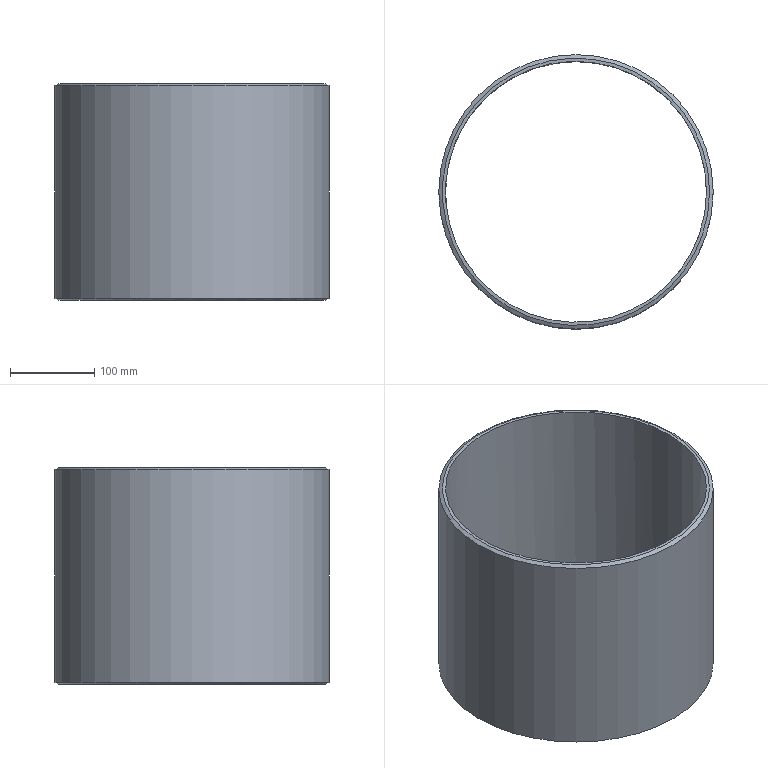Part | NX | features CHAMFER 1, CYLINDER 1, DATUM_CSYS 1, SHELL 1 | 1 solid | 6 faces | box 325 x 325 x 256.774 mm | volume 2034780 mm3 | plane 2 | cylinder 2 | cone 2 | commonest cylinder face diameters 309 x1 325 x1
STEP:
#1=CARTESIAN_POINT('',(158.17,0.,256.774));
#2=VERTEX_POINT('',#1);
#3=CARTESIAN_POINT('',(0.,0.,256.774));
#4=DIRECTION('',(0.,0.,1.));
#5=DIRECTION('',(1.,0.,0.));
#6=AXIS2_PLACEMENT_3D('',#3,#4,#5);
#7=CIRCLE('',#6,158.17);
#8=EDGE_CURVE('',#2,#2,#7,.T.);
#9=ORIENTED_EDGE('',*,*,#8,.T.);
#10=EDGE_LOOP('',(#9));
#11=FACE_BOUND('',#10,.T.);
#12=CARTESIAN_POINT('',(154.5,0.,256.774));
#13=VERTEX_POINT('',#12);
#14=CARTESIAN_POINT('',(0.,0.,256.774));
#15=DIRECTION('',(0.,0.,1.));
#16=DIRECTION('',(1.,0.,0.));
#17=AXIS2_PLACEMENT_3D('',#14,#15,#16);
#18=CIRCLE('',#17,154.5);
#19=EDGE_CURVE('',#13,#13,#18,.F.);
#20=ORIENTED_EDGE('',*,*,#19,.T.);
#21=EDGE_LOOP('',(#20));
#22=FACE_BOUND('',#21,.T.);
#23=CARTESIAN_POINT('',(0.,0.,256.774));
#24=DIRECTION('',(0.,0.,1.));
#25=DIRECTION('',(1.,0.,0.));
#26=AXIS2_PLACEMENT_3D('',#23,#24,#25);
#27=PLANE('',#26);
#28=ADVANCED_FACE('',(#11,#22),#27,.T.);
#29=CARTESIAN_POINT('',(-158.17,0.,0.));
#30=VERTEX_POINT('',#29);
#31=CARTESIAN_POINT('',(0.,0.,0.));
#32=DIRECTION('',(0.,0.,-1.));
#33=DIRECTION('',(-1.,0.,0.));
#34=AXIS2_PLACEMENT_3D('',#31,#32,#33);
#35=CIRCLE('',#34,158.17);
#36=EDGE_CURVE('',#30,#30,#35,.T.);
#37=ORIENTED_EDGE('',*,*,#36,.T.);
#38=EDGE_LOOP('',(#37));
#39=FACE_BOUND('',#38,.T.);
#40=CARTESIAN_POINT('',(-154.5,0.,0.));
#41=VERTEX_POINT('',#40);
#42=CARTESIAN_POINT('',(0.,0.,0.));
#43=DIRECTION('',(0.,0.,-1.));
#44=DIRECTION('',(-1.,0.,0.));
#45=AXIS2_PLACEMENT_3D('',#42,#43,#44);
#46=CIRCLE('',#45,154.5);
#47=EDGE_CURVE('',#41,#41,#46,.F.);
#48=ORIENTED_EDGE('',*,*,#47,.T.);
#49=EDGE_LOOP('',(#48));
#50=FACE_BOUND('',#49,.T.);
#51=CARTESIAN_POINT('',(0.,0.,0.));
#52=DIRECTION('',(0.,0.,-1.));
#53=DIRECTION('',(-1.,0.,0.));
#54=AXIS2_PLACEMENT_3D('',#51,#52,#53);
#55=PLANE('',#54);
#56=ADVANCED_FACE('',(#39,#50),#55,.T.);
#57=CARTESIAN_POINT('',(-162.5,0.,2.5));
#58=VERTEX_POINT('',#57);
#59=CARTESIAN_POINT('',(0.,0.,2.5));
#60=DIRECTION('',(0.,0.,-1.));
#61=DIRECTION('',(-1.,0.,0.));
#62=AXIS2_PLACEMENT_3D('',#59,#60,#61);
#63=CIRCLE('',#62,162.5);
#64=EDGE_CURVE('',#58,#58,#63,.F.);
#65=ORIENTED_EDGE('',*,*,#64,.T.);
#66=EDGE_LOOP('',(#65));
#67=FACE_BOUND('',#66,.T.);
#68=CARTESIAN_POINT('',(162.5,0.,254.274));
#69=VERTEX_POINT('',#68);
#70=CARTESIAN_POINT('',(0.,0.,254.274));
#71=DIRECTION('',(0.,0.,1.));
#72=DIRECTION('',(1.,0.,0.));
#73=AXIS2_PLACEMENT_3D('',#70,#71,#72);
#74=CIRCLE('',#73,162.5);
#75=EDGE_CURVE('',#69,#69,#74,.F.);
#76=ORIENTED_EDGE('',*,*,#75,.T.);
#77=EDGE_LOOP('',(#76));
#78=FACE_BOUND('',#77,.T.);
#79=CARTESIAN_POINT('',(0.,0.,0.));
#80=DIRECTION('',(0.,0.,1.));
#81=DIRECTION('',(1.,0.,0.));
#82=AXIS2_PLACEMENT_3D('',#79,#80,#81);
#83=CYLINDRICAL_SURFACE('',#82,162.5);
#84=ADVANCED_FACE('',(#67,#78),#83,.T.);
#85=ORIENTED_EDGE('',*,*,#19,.F.);
#86=EDGE_LOOP('',(#85));
#87=FACE_BOUND('',#86,.T.);
#88=ORIENTED_EDGE('',*,*,#47,.F.);
#89=EDGE_LOOP('',(#88));
#90=FACE_BOUND('',#89,.T.);
#91=CARTESIAN_POINT('',(0.,0.,0.));
#92=DIRECTION('',(0.,0.,1.));
#93=DIRECTION('',(1.,0.,0.));
#94=AXIS2_PLACEMENT_3D('',#91,#92,#93);
#95=CYLINDRICAL_SURFACE('',#94,154.5);
#96=ADVANCED_FACE('',(#87,#90),#95,.F.);
#97=ORIENTED_EDGE('',*,*,#36,.F.);
#98=EDGE_LOOP('',(#97));
#99=FACE_BOUND('',#98,.T.);
#100=ORIENTED_EDGE('',*,*,#64,.F.);
#101=EDGE_LOOP('',(#100));
#102=FACE_BOUND('',#101,.T.);
#103=CARTESIAN_POINT('',(0.,0.,2.5));
#104=DIRECTION('',(0.,0.,1.));
#105=DIRECTION('',(1.,0.,0.));
#106=AXIS2_PLACEMENT_3D('',#103,#104,#105);
#107=CONICAL_SURFACE('',#106,162.5,1.047);
#108=ADVANCED_FACE('',(#99,#102),#107,.T.);
#109=ORIENTED_EDGE('',*,*,#8,.F.);
#110=EDGE_LOOP('',(#109));
#111=FACE_BOUND('',#110,.T.);
#112=ORIENTED_EDGE('',*,*,#75,.F.);
#113=EDGE_LOOP('',(#112));
#114=FACE_BOUND('',#113,.T.);
#115=CARTESIAN_POINT('',(0.,0.,254.274));
#116=DIRECTION('',(0.,0.,-1.));
#117=DIRECTION('',(-1.,0.,0.));
#118=AXIS2_PLACEMENT_3D('',#115,#116,#117);
#119=CONICAL_SURFACE('',#118,162.5,1.047);
#120=ADVANCED_FACE('',(#111,#114),#119,.T.);
#121=CLOSED_SHELL('',(#28,#56,#84,#96,#108,#120));
#122=MANIFOLD_SOLID_BREP('',#121);
#123=(LENGTH_UNIT()NAMED_UNIT(*)SI_UNIT(.MILLI.,.METRE.));
#124=UNCERTAINTY_MEASURE_WITH_UNIT(LENGTH_MEASURE(0.00001),#123,'','');
#125=(NAMED_UNIT(*)PLANE_ANGLE_UNIT()SI_UNIT($,.RADIAN.));
#126=(NAMED_UNIT(*)SI_UNIT($,.STERADIAN.)SOLID_ANGLE_UNIT());
#127=(GEOMETRIC_REPRESENTATION_CONTEXT(3)GLOBAL_UNCERTAINTY_ASSIGNED_CONTEXT((#124))GLOBAL_UNIT_ASSIGNED_CONTEXT((#123,#125,#126))REPRESENTATION_CONTEXT('',''));
#128=ADVANCED_BREP_SHAPE_REPRESENTATION('',(#122),#127);